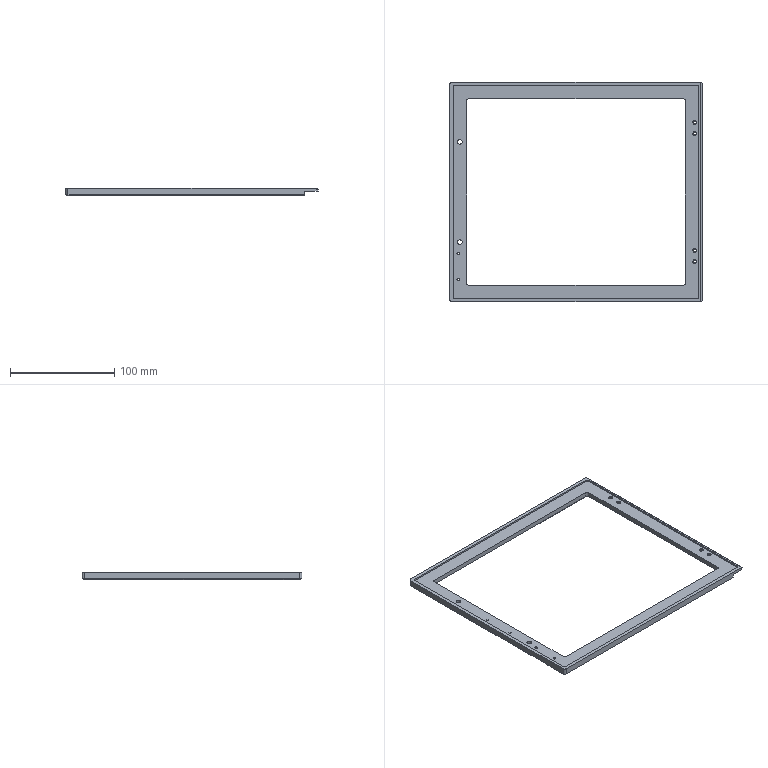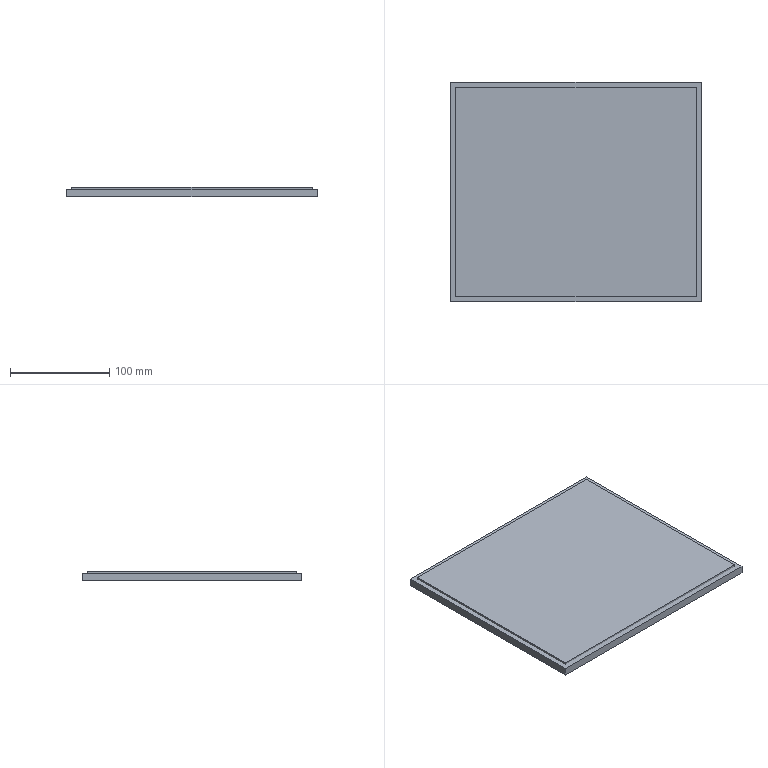CAM job | NX | 3-axis milling, drilling | part box 241.5 x 210.5 x 7 mm | stock box 251.5 x 220.5 x 10 mm
Tools:
number,name,description,diameter,corner_radius,flute_length,length,flutes
1,D63,Milling Tool-5 Parameters,63.0,0.0,50.0,75.0,2
10,D10,Milling Tool-5 Parameters,10.0,0.0,50.0,75.0,2
4,D4,Milling Tool-5 Parameters,4.0,0.0,50.0,75.0,2
7,D6A45,Milling Tool-5 Parameters,6.0,0.0,50.0,75.0,2
2,D2,Milling Tool-5 Parameters,2.0,0.0,50.0,75.0,2
6,D6,Milling Tool-5 Parameters,6.0,0.0,50.0,75.0,2
12,2.5ZT,Drilling Tool,2.5,0.0,35.0,50.0,2
14,4.5ZT,Drilling Tool,4.5,0.0,35.0,50.0,2
Operations:
program,operation,operation_type,tool,method,geometry_group,spindle_rpm,surface_speed,feed_per_tooth,feed_cut,feed_plunge,cut_length_mm,path_length_mm,cut_time_min,machine_time_min
1,FLOOR_WALL,VolumeBased25DMillingOperation,D63,METHOD,A,6500.0,122.0,0.1154,1500.0,100.0,1779.797,1833.797,1.187,1.192
1,ADAPTIVE_MILLING,CavityMilling,D10,METHOD,A,9500.0,298.0,0.1579,3000.0,1000.0,4738.321,4806.321,1.581,1.588
1,FLOOR_WALL_1,VolumeBased25DMillingOperation,D10,METHOD,A,9500.0,298.0,0.1316,2500.0,1000.0,13722.072,13879.279,5.539,5.555
1,FLOOR_WALL_1_COPY,VolumeBased25DMillingOperation,D10,METHOD,A,9500.0,298.0,0.0737,1400.0,1000.0,8679.306,8737.806,6.203,6.209
1,HOLE_MILLING,CylinderMilling,D10,METHOD,A,9500.0,298.0,0.1053,2000.0,100.0,317.639,1011.639,0.1588,0.2282
1,CAVITY_MILL,CavityMilling,D4,METHOD,A,9500.0,119.0,0.0789,1500.0,1000.0,180.148,1110.45,0.1294,0.2224
1,ZLEVEL_PROFILE,ZLevelMilling,D4,METHOD,A,9500.0,119.0,0.0737,1400.0,100.0,918.303,989.303,0.6559,0.663
1,ZLEVEL_PROFILE_1,ZLevelMilling,D2,METHOD,A,9500.0,59.0,0.0658,1250.0,100.0,543.482,927.02,0.4348,0.4731
1,PLANAR_MILL,PlanarMilling,D6A45,METHOD,A,9500.0,179.0,0.0658,1250.0,100.0,1785.892,1909.457,1.429,1.441
1,PLANAR_MILL_COPY_COPY,PlanarMilling,D6A45,METHOD,A,9500.0,179.0,0.0658,1250.0,100.0,430.237,766.144,0.3442,0.3778
2,FLOOR_WALL_COPY,VolumeBased25DMillingOperation,D10,METHOD,B,9500.0,298.0,0.1579,3000.0,800.0,7776.503,11238.276,2.667,3.014
2,FLOOR_WALL_COPY_COPY,VolumeBased25DMillingOperation,D10,METHOD,B,9500.0,298.0,0.0737,1400.0,800.0,2600.023,3534.2,1.876,1.969
2,FLOOR_WALL_2,VolumeBased25DMillingOperation,D6,METHOD,B,9500.0,179.0,0.1316,2500.0,1000.0,1191.928,1578.561,0.5777,0.6163
2,FLOOR_WALL_3,VolumeBased25DMillingOperation,D6,METHOD,B,9500.0,179.0,0.1316,2500.0,1000.0,5926.707,6820.195,2.398,2.487
2,FLOOR_WALL_3_COPY,VolumeBased25DMillingOperation,D6,METHOD,B,9500.0,179.0,0.1316,2500.0,1000.0,228.848,381.448,0.0952,0.1105
2,FLOOR_WALL_4,VolumeBased25DMillingOperation,D6,METHOD,B,9500.0,179.0,0.0658,1250.0,100.0,1560.896,2927.39,1.249,1.385
2,FLOOR_WALL_4_COPY,VolumeBased25DMillingOperation,D6,METHOD,B,9500.0,179.0,0.0658,1250.0,100.0,230.762,703.101,0.1846,0.2318
2,CAVITY_MILL_COPY,CavityMilling,D2,METHOD,B,9500.0,59.0,0.0579,1100.0,1000.0,646.153,2719.078,0.5978,0.8051
2,DRILLING,Operation,D6A45,METHOD,B,5000.0,94.0,0.025,250.0,0.0,23.0,459.458,0.092,0.1356
2,DRILLING_COPY,Operation,D6A45,METHOD,B,5000.0,94.0,0.025,250.0,0.0,8.7,203.55,0.0348,0.0543
2,DRILLING_COPY_COPY,Operation,2.5ZT,METHOD,B,2000.0,15.0,0.03,120.0,0.0,13.0,212.15,0.1083,0.1282
2,DRILLING_COPY_COPY_COPY_1,Operation,2.5ZT,METHOD,B,2000.0,15.0,0.03,120.0,0.0,18.702,218.384,0.1559,0.1758
2,DRILLING_COPY_COPY_COPY,Operation,4.5ZT,METHOD,B,2000.0,28.0,0.05,200.0,0.0,22.704,294.455,0.1135,0.1407
2,PLANAR_MILL_COPY_COPY_COPY,PlanarMilling,D6A45,METHOD,B,9500.0,179.0,0.0658,1250.0,900.0,1451.37,1976.487,1.165,1.217
2,PLANAR_MILL_COPY_COPY_COPY_COPY,PlanarMilling,D6A45,METHOD,B,9500.0,179.0,0.0658,1250.0,100.0,215.245,364.245,0.1722,0.1871
2,PLANAR_MILL_COPY_COPY_COPY_COPY_COPY,PlanarMilling,D6A45,METHOD,B,9500.0,179.0,0.0658,1250.0,100.0,237.066,394.866,0.1897,0.2054
2,ZLEVEL_PROFILE_1_COPY,ZLevelMilling,D6A45,METHOD,B,9500.0,59.0,0.0658,1250.0,100.0,386.027,783.932,0.3088,0.3486
2,ZLEVEL_PROFILE_2,ZLevelMilling,D4,METHOD,B,9500.0,119.0,0.0789,1500.0,100.0,12968.356,13122.856,8.646,8.661